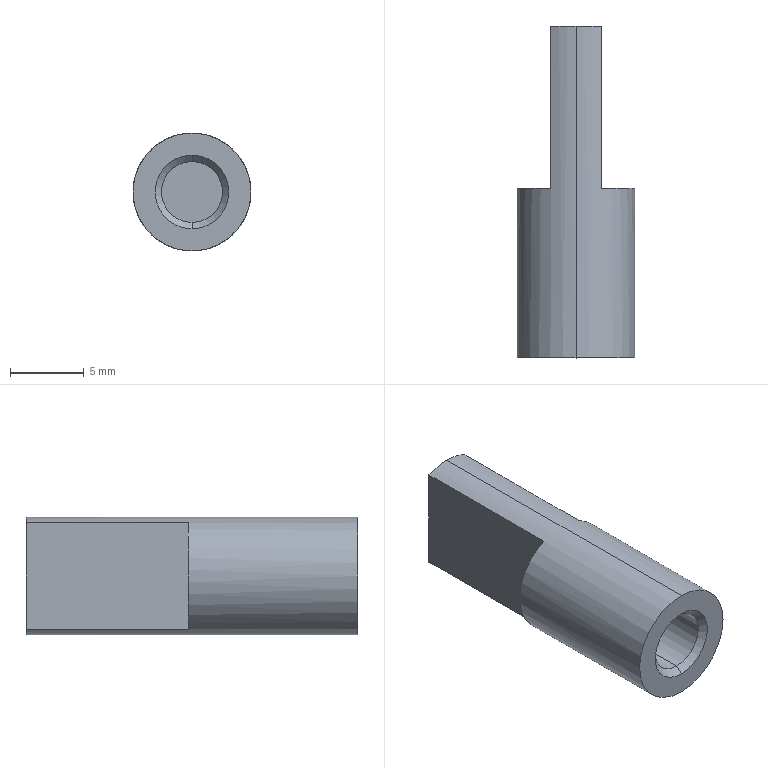Part | STEP file | HI_XAL51-D8-L100-H50-002^XAL51-D8-L100-H50 | 1 solid | 13 faces | box 8 x 22.5 x 8 mm | volume 786.148 mm3 | plane 7 | cylinder 4 | cone 2 | commonest cylinder face diameters 4.134 x2 8 x2
STEP:
#1=CARTESIAN_POINT('',(0.,0.,0.));
#2=DIRECTION('',(0.,0.,1.));
#3=DIRECTION('',(1.,0.,0.));
#4=AXIS2_PLACEMENT_3D('',#1,#2,#3);
#5=CARTESIAN_POINT('',(0.,0.,4.));
#6=VERTEX_POINT('',#5);
#7=CARTESIAN_POINT('',(0.,0.,-4.));
#8=VERTEX_POINT('',#7);
#9=CARTESIAN_POINT('',(0.,0.,0.));
#10=DIRECTION('',(0.,-1.,0.));
#11=DIRECTION('',(0.,0.,-1.));
#12=AXIS2_PLACEMENT_3D('',#9,#10,#11);
#13=CIRCLE('',#12,4.);
#14=CARTESIAN_POINT('',(0.,0.,0.));
#15=DIRECTION('',(0.,1.,0.));
#16=DIRECTION('',(0.,0.,-1.));
#17=AXIS2_PLACEMENT_3D('',#14,#15,#16);
#18=CYLINDRICAL_SURFACE('',#17,4.);
#19=CARTESIAN_POINT('',(6.283,0.));
#20=DIRECTION('',(-1.,0.));
#21=VECTOR('',#20,1.);
#22=LINE('',#19,#21);
#23=(GEOMETRIC_REPRESENTATION_CONTEXT(2)PARAMETRIC_REPRESENTATION_CONTEXT()REPRESENTATION_CONTEXT('',''));
#24=DEFINITIONAL_REPRESENTATION('',(#22),#23);
#25=PCURVE('',#18,#24);
#26=CARTESIAN_POINT('',(4.,0.,0.));
#27=DIRECTION('',(0.,1.,0.));
#28=DIRECTION('',(1.,0.,0.));
#29=AXIS2_PLACEMENT_3D('',#26,#27,#28);
#30=PLANE('',#29);
#31=CARTESIAN_POINT('',(-4.,4.));
#32=CARTESIAN_POINT('',(2.928,4.));
#33=CARTESIAN_POINT('',(-0.5359,-2.));
#34=CARTESIAN_POINT('',(-4.,-8.));
#35=CARTESIAN_POINT('',(-7.464,-2.));
#36=CARTESIAN_POINT('',(-10.928,4.));
#37=CARTESIAN_POINT('',(-4.,4.));
#38=(BOUNDED_CURVE()B_SPLINE_CURVE(2,(#31,#32,#33,#34,#35,#36,#37),.UNSPECIFIED.,.T.,.F.)B_SPLINE_CURVE_WITH_KNOTS((1,2,2,2,2,1),(-2.094,0.,2.094,4.189,6.283,8.378),.UNSPECIFIED.)CURVE()GEOMETRIC_REPRESENTATION_ITEM()RATIONAL_B_SPLINE_CURVE((1.,0.5,1.,0.5,1.,0.5,1.))REPRESENTATION_ITEM(''));
#39=(GEOMETRIC_REPRESENTATION_CONTEXT(2)PARAMETRIC_REPRESENTATION_CONTEXT()REPRESENTATION_CONTEXT('',''));
#40=DEFINITIONAL_REPRESENTATION('',(#38),#39);
#41=PCURVE('',#30,#40);
#42=SURFACE_CURVE('',#13,(#25,#41),.PCURVE_S1.);
#43=EDGE_CURVE('',#6,#8,#42,.T.);
#44=ORIENTED_EDGE('',*,*,#43,.F.);
#45=CARTESIAN_POINT('',(0.,22.5,4.));
#46=VERTEX_POINT('',#45);
#47=CARTESIAN_POINT('',(0.,0.,4.));
#48=DIRECTION('',(0.,1.,0.));
#49=VECTOR('',#48,1.);
#50=LINE('',#47,#49);
#51=CARTESIAN_POINT('',(3.142,0.));
#52=DIRECTION('',(0.,1.));
#53=VECTOR('',#52,1.);
#54=LINE('',#51,#53);
#55=(GEOMETRIC_REPRESENTATION_CONTEXT(2)PARAMETRIC_REPRESENTATION_CONTEXT()REPRESENTATION_CONTEXT('',''));
#56=DEFINITIONAL_REPRESENTATION('',(#54),#55);
#57=PCURVE('',#18,#56);
#58=CARTESIAN_POINT('',(0.,0.,0.));
#59=DIRECTION('',(0.,1.,0.));
#60=DIRECTION('',(0.,0.,-1.));
#61=AXIS2_PLACEMENT_3D('',#58,#59,#60);
#62=CYLINDRICAL_SURFACE('',#61,4.);
#63=CARTESIAN_POINT('',(3.142,0.));
#64=DIRECTION('',(0.,1.));
#65=VECTOR('',#64,1.);
#66=LINE('',#63,#65);
#67=(GEOMETRIC_REPRESENTATION_CONTEXT(2)PARAMETRIC_REPRESENTATION_CONTEXT()REPRESENTATION_CONTEXT('',''));
#68=DEFINITIONAL_REPRESENTATION('',(#66),#67);
#69=PCURVE('',#62,#68);
#70=SURFACE_CURVE('',#50,(#57,#69),.PCURVE_S1.);
#71=EDGE_CURVE('',#6,#46,#70,.T.);
#72=ORIENTED_EDGE('',*,*,#71,.T.);
#73=CARTESIAN_POINT('',(-1.7,22.5,3.621));
#74=VERTEX_POINT('',#73);
#75=CARTESIAN_POINT('',(0.,22.5,0.));
#76=DIRECTION('',(0.,-1.,0.));
#77=DIRECTION('',(0.,0.,-1.));
#78=AXIS2_PLACEMENT_3D('',#75,#76,#77);
#79=CIRCLE('',#78,4.);
#80=CARTESIAN_POINT('',(6.283,22.5));
#81=DIRECTION('',(-1.,0.));
#82=VECTOR('',#81,1.);
#83=LINE('',#80,#82);
#84=(GEOMETRIC_REPRESENTATION_CONTEXT(2)PARAMETRIC_REPRESENTATION_CONTEXT()REPRESENTATION_CONTEXT('',''));
#85=DEFINITIONAL_REPRESENTATION('',(#83),#84);
#86=PCURVE('',#18,#85);
#87=CARTESIAN_POINT('',(0.,22.5,0.));
#88=DIRECTION('',(0.,-1.,0.));
#89=DIRECTION('',(0.,0.,-1.));
#90=AXIS2_PLACEMENT_3D('',#87,#88,#89);
#91=PLANE('',#90);
#92=CARTESIAN_POINT('',(0.,0.));
#93=DIRECTION('',(1.,0.));
#94=AXIS2_PLACEMENT_2D('',#92,#93);
#95=CIRCLE('',#94,4.);
#96=(GEOMETRIC_REPRESENTATION_CONTEXT(2)PARAMETRIC_REPRESENTATION_CONTEXT()REPRESENTATION_CONTEXT('',''));
#97=DEFINITIONAL_REPRESENTATION('',(#95),#96);
#98=PCURVE('',#91,#97);
#99=SURFACE_CURVE('',#79,(#86,#98),.PCURVE_S1.);
#100=EDGE_CURVE('',#46,#74,#99,.T.);
#101=ORIENTED_EDGE('',*,*,#100,.T.);
#102=CARTESIAN_POINT('',(-1.7,11.5,3.621));
#103=VERTEX_POINT('',#102);
#104=CARTESIAN_POINT('',(-1.7,0.,3.621));
#105=DIRECTION('',(0.,1.,0.));
#106=VECTOR('',#105,1.);
#107=LINE('',#104,#106);
#108=CARTESIAN_POINT('',(2.703,0.));
#109=DIRECTION('',(0.,1.));
#110=VECTOR('',#109,1.);
#111=LINE('',#108,#110);
#112=(GEOMETRIC_REPRESENTATION_CONTEXT(2)PARAMETRIC_REPRESENTATION_CONTEXT()REPRESENTATION_CONTEXT('',''));
#113=DEFINITIONAL_REPRESENTATION('',(#111),#112);
#114=PCURVE('',#18,#113);
#115=CARTESIAN_POINT('',(-1.7,11.5,8.));
#116=DIRECTION('',(-1.,0.,0.));
#117=DIRECTION('',(0.,0.,1.));
#118=AXIS2_PLACEMENT_3D('',#115,#116,#117);
#119=PLANE('',#118);
#120=CARTESIAN_POINT('',(-4.379,-11.5));
#121=DIRECTION('',(0.,1.));
#122=VECTOR('',#121,1.);
#123=LINE('',#120,#122);
#124=(GEOMETRIC_REPRESENTATION_CONTEXT(2)PARAMETRIC_REPRESENTATION_CONTEXT()REPRESENTATION_CONTEXT('',''));
#125=DEFINITIONAL_REPRESENTATION('',(#123),#124);
#126=PCURVE('',#119,#125);
#127=SURFACE_CURVE('',#107,(#114,#126),.PCURVE_S1.);
#128=EDGE_CURVE('',#103,#74,#127,.T.);
#129=ORIENTED_EDGE('',*,*,#128,.F.);
#130=CARTESIAN_POINT('',(-1.7,11.5,-3.621));
#131=VERTEX_POINT('',#130);
#132=CARTESIAN_POINT('',(0.,11.5,0.));
#133=DIRECTION('',(0.,1.,0.));
#134=DIRECTION('',(0.,0.,1.));
#135=AXIS2_PLACEMENT_3D('',#132,#133,#134);
#136=CIRCLE('',#135,4.);
#137=CARTESIAN_POINT('',(-3.142,11.5));
#138=DIRECTION('',(1.,0.));
#139=VECTOR('',#138,1.);
#140=LINE('',#137,#139);
#141=(GEOMETRIC_REPRESENTATION_CONTEXT(2)PARAMETRIC_REPRESENTATION_CONTEXT()REPRESENTATION_CONTEXT('',''));
#142=DEFINITIONAL_REPRESENTATION('',(#140),#141);
#143=PCURVE('',#18,#142);
#144=CARTESIAN_POINT('',(-9.7,11.5,8.));
#145=DIRECTION('',(0.,1.,0.));
#146=DIRECTION('',(1.,0.,0.));
#147=AXIS2_PLACEMENT_3D('',#144,#145,#146);
#148=PLANE('',#147);
#149=CARTESIAN_POINT('',(9.7,8.));
#150=DIRECTION('',(0.,-1.));
#151=AXIS2_PLACEMENT_2D('',#149,#150);
#152=CIRCLE('',#151,4.);
#153=(GEOMETRIC_REPRESENTATION_CONTEXT(2)PARAMETRIC_REPRESENTATION_CONTEXT()REPRESENTATION_CONTEXT('',''));
#154=DEFINITIONAL_REPRESENTATION('',(#152),#153);
#155=PCURVE('',#148,#154);
#156=SURFACE_CURVE('',#136,(#143,#155),.PCURVE_S1.);
#157=EDGE_CURVE('',#131,#103,#156,.T.);
#158=ORIENTED_EDGE('',*,*,#157,.F.);
#159=CARTESIAN_POINT('',(-1.7,22.5,-3.621));
#160=VERTEX_POINT('',#159);
#161=CARTESIAN_POINT('',(-1.7,0.,-3.621));
#162=DIRECTION('',(0.,-1.,0.));
#163=VECTOR('',#162,1.);
#164=LINE('',#161,#163);
#165=CARTESIAN_POINT('',(0.439,0.));
#166=DIRECTION('',(0.,-1.));
#167=VECTOR('',#166,1.);
#168=LINE('',#165,#167);
#169=(GEOMETRIC_REPRESENTATION_CONTEXT(2)PARAMETRIC_REPRESENTATION_CONTEXT()REPRESENTATION_CONTEXT('',''));
#170=DEFINITIONAL_REPRESENTATION('',(#168),#169);
#171=PCURVE('',#18,#170);
#172=CARTESIAN_POINT('',(-11.621,-11.5));
#173=DIRECTION('',(0.,-1.));
#174=VECTOR('',#173,1.);
#175=LINE('',#172,#174);
#176=(GEOMETRIC_REPRESENTATION_CONTEXT(2)PARAMETRIC_REPRESENTATION_CONTEXT()REPRESENTATION_CONTEXT('',''));
#177=DEFINITIONAL_REPRESENTATION('',(#175),#176);
#178=PCURVE('',#119,#177);
#179=SURFACE_CURVE('',#164,(#171,#178),.PCURVE_S1.);
#180=EDGE_CURVE('',#160,#131,#179,.T.);
#181=ORIENTED_EDGE('',*,*,#180,.F.);
#182=CARTESIAN_POINT('',(0.,22.5,-4.));
#183=VERTEX_POINT('',#182);
#184=CARTESIAN_POINT('',(0.,22.5,0.));
#185=DIRECTION('',(0.,-1.,0.));
#186=DIRECTION('',(0.,0.,-1.));
#187=AXIS2_PLACEMENT_3D('',#184,#185,#186);
#188=CIRCLE('',#187,4.);
#189=CARTESIAN_POINT('',(6.283,22.5));
#190=DIRECTION('',(-1.,0.));
#191=VECTOR('',#190,1.);
#192=LINE('',#189,#191);
#193=(GEOMETRIC_REPRESENTATION_CONTEXT(2)PARAMETRIC_REPRESENTATION_CONTEXT()REPRESENTATION_CONTEXT('',''));
#194=DEFINITIONAL_REPRESENTATION('',(#192),#193);
#195=PCURVE('',#18,#194);
#196=CARTESIAN_POINT('',(0.,0.));
#197=DIRECTION('',(1.,0.));
#198=AXIS2_PLACEMENT_2D('',#196,#197);
#199=CIRCLE('',#198,4.);
#200=(GEOMETRIC_REPRESENTATION_CONTEXT(2)PARAMETRIC_REPRESENTATION_CONTEXT()REPRESENTATION_CONTEXT('',''));
#201=DEFINITIONAL_REPRESENTATION('',(#199),#200);
#202=PCURVE('',#91,#201);
#203=SURFACE_CURVE('',#188,(#195,#202),.PCURVE_S1.);
#204=EDGE_CURVE('',#160,#183,#203,.T.);
#205=ORIENTED_EDGE('',*,*,#204,.T.);
#206=CARTESIAN_POINT('',(0.,0.,-4.));
#207=DIRECTION('',(0.,1.,0.));
#208=VECTOR('',#207,1.);
#209=LINE('',#206,#208);
#210=CARTESIAN_POINT('',(0.,0.));
#211=DIRECTION('',(0.,1.));
#212=VECTOR('',#211,1.);
#213=LINE('',#210,#212);
#214=(GEOMETRIC_REPRESENTATION_CONTEXT(2)PARAMETRIC_REPRESENTATION_CONTEXT()REPRESENTATION_CONTEXT('',''));
#215=DEFINITIONAL_REPRESENTATION('',(#213),#214);
#216=PCURVE('',#18,#215);
#217=CARTESIAN_POINT('',(6.283,0.));
#218=DIRECTION('',(0.,1.));
#219=VECTOR('',#218,1.);
#220=LINE('',#217,#219);
#221=(GEOMETRIC_REPRESENTATION_CONTEXT(2)PARAMETRIC_REPRESENTATION_CONTEXT()REPRESENTATION_CONTEXT('',''));
#222=DEFINITIONAL_REPRESENTATION('',(#220),#221);
#223=PCURVE('',#62,#222);
#224=SURFACE_CURVE('',#209,(#216,#223),.PCURVE_S1.);
#225=EDGE_CURVE('',#8,#183,#224,.T.);
#226=ORIENTED_EDGE('',*,*,#225,.F.);
#227=EDGE_LOOP('',(#44,#72,#101,#129,#158,#181,#205,#226));
#228=FACE_BOUND('',#227,.T.);
#229=ADVANCED_FACE('',(#228),#18,.T.);
#230=CARTESIAN_POINT('',(0.,0.433,-2.067));
#231=VERTEX_POINT('',#230);
#232=CARTESIAN_POINT('',(0.,0.,-2.5));
#233=VERTEX_POINT('',#232);
#234=CARTESIAN_POINT('',(0.,0.433,-2.067));
#235=DIRECTION('',(0.,-0.7071,-0.7071));
#236=VECTOR('',#235,1.);
#237=LINE('',#234,#236);
#238=CARTESIAN_POINT('',(0.,0.433,0.));
#239=DIRECTION('',(0.,-1.,0.));
#240=DIRECTION('',(0.,0.,-1.));
#241=AXIS2_PLACEMENT_3D('',#238,#239,#240);
#242=CONICAL_SURFACE('',#241,2.067,0.7854);
#243=CARTESIAN_POINT('',(6.283,0.));
#244=DIRECTION('',(0.,1.));
#245=VECTOR('',#244,1.);
#246=LINE('',#243,#245);
#247=(GEOMETRIC_REPRESENTATION_CONTEXT(2)PARAMETRIC_REPRESENTATION_CONTEXT()REPRESENTATION_CONTEXT('',''));
#248=DEFINITIONAL_REPRESENTATION('',(#246),#247);
#249=PCURVE('',#242,#248);
#250=CARTESIAN_POINT('',(0.,0.433,0.));
#251=DIRECTION('',(0.,-1.,0.));
#252=DIRECTION('',(0.,0.,-1.));
#253=AXIS2_PLACEMENT_3D('',#250,#251,#252);
#254=CONICAL_SURFACE('',#253,2.067,0.7854);
#255=CARTESIAN_POINT('',(0.,0.));
#256=DIRECTION('',(0.,1.));
#257=VECTOR('',#256,1.);
#258=LINE('',#255,#257);
#259=(GEOMETRIC_REPRESENTATION_CONTEXT(2)PARAMETRIC_REPRESENTATION_CONTEXT()REPRESENTATION_CONTEXT('',''));
#260=DEFINITIONAL_REPRESENTATION('',(#258),#259);
#261=PCURVE('',#254,#260);
#262=SURFACE_CURVE('',#237,(#249,#261),.PCURVE_S1.);
#263=EDGE_CURVE('',#231,#233,#262,.T.);
#264=ORIENTED_EDGE('',*,*,#263,.T.);
#265=CARTESIAN_POINT('',(0.,0.,2.5));
#266=VERTEX_POINT('',#265);
#267=CARTESIAN_POINT('',(0.,0.,0.));
#268=DIRECTION('',(0.,-1.,0.));
#269=DIRECTION('',(0.,0.,-1.));
#270=AXIS2_PLACEMENT_3D('',#267,#268,#269);
#271=CIRCLE('',#270,2.5);
#272=CARTESIAN_POINT('',(0.,0.433));
#273=DIRECTION('',(1.,0.));
#274=VECTOR('',#273,1.);
#275=LINE('',#272,#274);
#276=(GEOMETRIC_REPRESENTATION_CONTEXT(2)PARAMETRIC_REPRESENTATION_CONTEXT()REPRESENTATION_CONTEXT('',''));
#277=DEFINITIONAL_REPRESENTATION('',(#275),#276);
#278=PCURVE('',#242,#277);
#279=CARTESIAN_POINT('',(-4.,2.5));
#280=CARTESIAN_POINT('',(0.3301,2.5));
#281=CARTESIAN_POINT('',(-1.835,-1.25));
#282=CARTESIAN_POINT('',(-4.,-5.));
#283=CARTESIAN_POINT('',(-6.165,-1.25));
#284=CARTESIAN_POINT('',(-8.33,2.5));
#285=CARTESIAN_POINT('',(-4.,2.5));
#286=(BOUNDED_CURVE()B_SPLINE_CURVE(2,(#279,#280,#281,#282,#283,#284,#285),.UNSPECIFIED.,.T.,.F.)B_SPLINE_CURVE_WITH_KNOTS((1,2,2,2,2,1),(-2.094,0.,2.094,4.189,6.283,8.378),.UNSPECIFIED.)CURVE()GEOMETRIC_REPRESENTATION_ITEM()RATIONAL_B_SPLINE_CURVE((1.,0.5,1.,0.5,1.,0.5,1.))REPRESENTATION_ITEM(''));
#287=(GEOMETRIC_REPRESENTATION_CONTEXT(2)PARAMETRIC_REPRESENTATION_CONTEXT()REPRESENTATION_CONTEXT('',''));
#288=DEFINITIONAL_REPRESENTATION('',(#286),#287);
#289=PCURVE('',#30,#288);
#290=SURFACE_CURVE('',#271,(#278,#289),.PCURVE_S1.);
#291=EDGE_CURVE('',#266,#233,#290,.T.);
#292=ORIENTED_EDGE('',*,*,#291,.F.);
#293=CARTESIAN_POINT('',(0.,0.433,2.067));
#294=VERTEX_POINT('',#293);
#295=CARTESIAN_POINT('',(0.,0.433,2.067));
#296=DIRECTION('',(0.,-0.7071,0.7071));
#297=VECTOR('',#296,1.);
#298=LINE('',#295,#297);
#299=CARTESIAN_POINT('',(3.142,0.));
#300=DIRECTION('',(0.,1.));
#301=VECTOR('',#300,1.);
#302=LINE('',#299,#301);
#303=(GEOMETRIC_REPRESENTATION_CONTEXT(2)PARAMETRIC_REPRESENTATION_CONTEXT()REPRESENTATION_CONTEXT('',''));
#304=DEFINITIONAL_REPRESENTATION('',(#302),#303);
#305=PCURVE('',#242,#304);
#306=CARTESIAN_POINT('',(3.142,0.));
#307=DIRECTION('',(0.,1.));
#308=VECTOR('',#307,1.);
#309=LINE('',#306,#308);
#310=(GEOMETRIC_REPRESENTATION_CONTEXT(2)PARAMETRIC_REPRESENTATION_CONTEXT()REPRESENTATION_CONTEXT('',''));
#311=DEFINITIONAL_REPRESENTATION('',(#309),#310);
#312=PCURVE('',#254,#311);
#313=SURFACE_CURVE('',#298,(#305,#312),.PCURVE_S1.);
#314=EDGE_CURVE('',#294,#266,#313,.T.);
#315=ORIENTED_EDGE('',*,*,#314,.F.);
#316=CARTESIAN_POINT('',(0.,0.433,0.));
#317=DIRECTION('',(0.,-1.,0.));
#318=DIRECTION('',(0.,0.,-1.));
#319=AXIS2_PLACEMENT_3D('',#316,#317,#318);
#320=CIRCLE('',#319,2.067);
#321=CARTESIAN_POINT('',(0.,0.));
#322=DIRECTION('',(1.,0.));
#323=VECTOR('',#322,1.);
#324=LINE('',#321,#323);
#325=(GEOMETRIC_REPRESENTATION_CONTEXT(2)PARAMETRIC_REPRESENTATION_CONTEXT()REPRESENTATION_CONTEXT('',''));
#326=DEFINITIONAL_REPRESENTATION('',(#324),#325);
#327=PCURVE('',#242,#326);
#328=CARTESIAN_POINT('',(0.,0.,0.));
#329=DIRECTION('',(0.,1.,0.));
#330=DIRECTION('',(0.,0.,-1.));
#331=AXIS2_PLACEMENT_3D('',#328,#329,#330);
#332=CYLINDRICAL_SURFACE('',#331,2.067);
#333=CARTESIAN_POINT('',(6.283,0.433));
#334=DIRECTION('',(-1.,0.));
#335=VECTOR('',#334,1.);
#336=LINE('',#333,#335);
#337=(GEOMETRIC_REPRESENTATION_CONTEXT(2)PARAMETRIC_REPRESENTATION_CONTEXT()REPRESENTATION_CONTEXT('',''));
#338=DEFINITIONAL_REPRESENTATION('',(#336),#337);
#339=PCURVE('',#332,#338);
#340=SURFACE_CURVE('',#320,(#327,#339),.PCURVE_S1.);
#341=EDGE_CURVE('',#294,#231,#340,.T.);
#342=ORIENTED_EDGE('',*,*,#341,.T.);
#343=EDGE_LOOP('',(#264,#292,#315,#342));
#344=FACE_BOUND('',#343,.F.);
#345=ADVANCED_FACE('',(#344),#242,.F.);
#346=CARTESIAN_POINT('',(0.,6.,-2.067));
#347=VERTEX_POINT('',#346);
#348=CARTESIAN_POINT('',(0.,0.,-2.067));
#349=DIRECTION('',(0.,1.,0.));
#350=VECTOR('',#349,1.);
#351=LINE('',#348,#350);
#352=CARTESIAN_POINT('',(0.,0.,0.));
#353=DIRECTION('',(0.,1.,0.));
#354=DIRECTION('',(0.,0.,-1.));
#355=AXIS2_PLACEMENT_3D('',#352,#353,#354);
#356=CYLINDRICAL_SURFACE('',#355,2.067);
#357=CARTESIAN_POINT('',(6.283,0.));
#358=DIRECTION('',(0.,1.));
#359=VECTOR('',#358,1.);
#360=LINE('',#357,#359);
#361=(GEOMETRIC_REPRESENTATION_CONTEXT(2)PARAMETRIC_REPRESENTATION_CONTEXT()REPRESENTATION_CONTEXT('',''));
#362=DEFINITIONAL_REPRESENTATION('',(#360),#361);
#363=PCURVE('',#356,#362);
#364=CARTESIAN_POINT('',(0.,0.));
#365=DIRECTION('',(0.,1.));
#366=VECTOR('',#365,1.);
#367=LINE('',#364,#366);
#368=(GEOMETRIC_REPRESENTATION_CONTEXT(2)PARAMETRIC_REPRESENTATION_CONTEXT()REPRESENTATION_CONTEXT('',''));
#369=DEFINITIONAL_REPRESENTATION('',(#367),#368);
#370=PCURVE('',#332,#369);
#371=SURFACE_CURVE('',#351,(#363,#370),.PCURVE_S1.);
#372=EDGE_CURVE('',#231,#347,#371,.T.);
#373=ORIENTED_EDGE('',*,*,#372,.T.);
#374=CARTESIAN_POINT('',(0.,6.,2.067));
#375=VERTEX_POINT('',#374);
#376=CARTESIAN_POINT('',(0.,6.,0.));
#377=DIRECTION('',(0.,-1.,0.));
#378=DIRECTION('',(0.,0.,-1.));
#379=AXIS2_PLACEMENT_3D('',#376,#377,#378);
#380=CIRCLE('',#379,2.067);
#381=CARTESIAN_POINT('',(6.283,6.));
#382=DIRECTION('',(-1.,0.));
#383=VECTOR('',#382,1.);
#384=LINE('',#381,#383);
#385=(GEOMETRIC_REPRESENTATION_CONTEXT(2)PARAMETRIC_REPRESENTATION_CONTEXT()REPRESENTATION_CONTEXT('',''));
#386=DEFINITIONAL_REPRESENTATION('',(#384),#385);
#387=PCURVE('',#356,#386);
#388=CARTESIAN_POINT('',(0.,6.,0.));
#389=DIRECTION('',(0.,-1.,0.));
#390=DIRECTION('',(0.,0.,-1.));
#391=AXIS2_PLACEMENT_3D('',#388,#389,#390);
#392=PLANE('',#391);
#393=CARTESIAN_POINT('',(0.,0.));
#394=DIRECTION('',(1.,0.));
#395=AXIS2_PLACEMENT_2D('',#393,#394);
#396=CIRCLE('',#395,2.067);
#397=(GEOMETRIC_REPRESENTATION_CONTEXT(2)PARAMETRIC_REPRESENTATION_CONTEXT()REPRESENTATION_CONTEXT('',''));
#398=DEFINITIONAL_REPRESENTATION('',(#396),#397);
#399=PCURVE('',#392,#398);
#400=SURFACE_CURVE('',#380,(#387,#399),.PCURVE_S1.);
#401=EDGE_CURVE('',#347,#375,#400,.T.);
#402=ORIENTED_EDGE('',*,*,#401,.T.);
#403=CARTESIAN_POINT('',(0.,0.,2.067));
#404=DIRECTION('',(0.,1.,0.));
#405=VECTOR('',#404,1.);
#406=LINE('',#403,#405);
#407=CARTESIAN_POINT('',(3.142,0.));
#408=DIRECTION('',(0.,1.));
#409=VECTOR('',#408,1.);
#410=LINE('',#407,#409);
#411=(GEOMETRIC_REPRESENTATION_CONTEXT(2)PARAMETRIC_REPRESENTATION_CONTEXT()REPRESENTATION_CONTEXT('',''));
#412=DEFINITIONAL_REPRESENTATION('',(#410),#411);
#413=PCURVE('',#356,#412);
#414=CARTESIAN_POINT('',(3.142,0.));
#415=DIRECTION('',(0.,1.));
#416=VECTOR('',#415,1.);
#417=LINE('',#414,#416);
#418=(GEOMETRIC_REPRESENTATION_CONTEXT(2)PARAMETRIC_REPRESENTATION_CONTEXT()REPRESENTATION_CONTEXT('',''));
#419=DEFINITIONAL_REPRESENTATION('',(#417),#418);
#420=PCURVE('',#332,#419);
#421=SURFACE_CURVE('',#406,(#413,#420),.PCURVE_S1.);
#422=EDGE_CURVE('',#294,#375,#421,.T.);
#423=ORIENTED_EDGE('',*,*,#422,.F.);
#424=CARTESIAN_POINT('',(0.,0.433,0.));
#425=DIRECTION('',(0.,-1.,0.));
#426=DIRECTION('',(0.,0.,-1.));
#427=AXIS2_PLACEMENT_3D('',#424,#425,#426);
#428=CIRCLE('',#427,2.067);
#429=CARTESIAN_POINT('',(6.283,0.433));
#430=DIRECTION('',(-1.,0.));
#431=VECTOR('',#430,1.);
#432=LINE('',#429,#431);
#433=(GEOMETRIC_REPRESENTATION_CONTEXT(2)PARAMETRIC_REPRESENTATION_CONTEXT()REPRESENTATION_CONTEXT('',''));
#434=DEFINITIONAL_REPRESENTATION('',(#432),#433);
#435=PCURVE('',#356,#434);
#436=CARTESIAN_POINT('',(0.,0.));
#437=DIRECTION('',(1.,0.));
#438=VECTOR('',#437,1.);
#439=LINE('',#436,#438);
#440=(GEOMETRIC_REPRESENTATION_CONTEXT(2)PARAMETRIC_REPRESENTATION_CONTEXT()REPRESENTATION_CONTEXT('',''));
#441=DEFINITIONAL_REPRESENTATION('',(#439),#440);
#442=PCURVE('',#254,#441);
#443=SURFACE_CURVE('',#428,(#435,#442),.PCURVE_S1.);
#444=EDGE_CURVE('',#231,#294,#443,.T.);
#445=ORIENTED_EDGE('',*,*,#444,.F.);
#446=EDGE_LOOP('',(#373,#402,#423,#445));
#447=FACE_BOUND('',#446,.F.);
#448=ADVANCED_FACE('',(#447),#356,.F.);
#449=ORIENTED_EDGE('',*,*,#401,.T.);
#450=CARTESIAN_POINT('',(0.,6.,0.));
#451=DIRECTION('',(0.,-1.,0.));
#452=DIRECTION('',(0.,0.,-1.));
#453=AXIS2_PLACEMENT_3D('',#450,#451,#452);
#454=CIRCLE('',#453,2.067);
#455=CARTESIAN_POINT('',(0.,0.));
#456=DIRECTION('',(1.,0.));
#457=AXIS2_PLACEMENT_2D('',#455,#456);
#458=CIRCLE('',#457,2.067);
#459=(GEOMETRIC_REPRESENTATION_CONTEXT(2)PARAMETRIC_REPRESENTATION_CONTEXT()REPRESENTATION_CONTEXT('',''));
#460=DEFINITIONAL_REPRESENTATION('',(#458),#459);
#461=PCURVE('',#392,#460);
#462=CARTESIAN_POINT('',(6.283,6.));
#463=DIRECTION('',(-1.,0.));
#464=VECTOR('',#463,1.);
#465=LINE('',#462,#464);
#466=(GEOMETRIC_REPRESENTATION_CONTEXT(2)PARAMETRIC_REPRESENTATION_CONTEXT()REPRESENTATION_CONTEXT('',''));
#467=DEFINITIONAL_REPRESENTATION('',(#465),#466);
#468=PCURVE('',#332,#467);
#469=SURFACE_CURVE('',#454,(#461,#468),.PCURVE_S1.);
#470=EDGE_CURVE('',#375,#347,#469,.T.);
#471=ORIENTED_EDGE('',*,*,#470,.T.);
#472=EDGE_LOOP('',(#449,#471));
#473=FACE_BOUND('',#472,.T.);
#474=ADVANCED_FACE('',(#473),#392,.T.);
#475=CARTESIAN_POINT('',(0.,0.,0.));
#476=DIRECTION('',(0.,-1.,0.));
#477=DIRECTION('',(0.,0.,-1.));
#478=AXIS2_PLACEMENT_3D('',#475,#476,#477);
#479=CIRCLE('',#478,2.5);
#480=CARTESIAN_POINT('',(-4.,2.5));
#481=CARTESIAN_POINT('',(0.3301,2.5));
#482=CARTESIAN_POINT('',(-1.835,-1.25));
#483=CARTESIAN_POINT('',(-4.,-5.));
#484=CARTESIAN_POINT('',(-6.165,-1.25));
#485=CARTESIAN_POINT('',(-8.33,2.5));
#486=CARTESIAN_POINT('',(-4.,2.5));
#487=(BOUNDED_CURVE()B_SPLINE_CURVE(2,(#480,#481,#482,#483,#484,#485,#486),.UNSPECIFIED.,.T.,.F.)B_SPLINE_CURVE_WITH_KNOTS((1,2,2,2,2,1),(-2.094,0.,2.094,4.189,6.283,8.378),.UNSPECIFIED.)CURVE()GEOMETRIC_REPRESENTATION_ITEM()RATIONAL_B_SPLINE_CURVE((1.,0.5,1.,0.5,1.,0.5,1.))REPRESENTATION_ITEM(''));
#488=(GEOMETRIC_REPRESENTATION_CONTEXT(2)PARAMETRIC_REPRESENTATION_CONTEXT()REPRESENTATION_CONTEXT('',''));
#489=DEFINITIONAL_REPRESENTATION('',(#487),#488);
#490=PCURVE('',#30,#489);
#491=CARTESIAN_POINT('',(0.,0.433));
#492=DIRECTION('',(1.,0.));
#493=VECTOR('',#492,1.);
#494=LINE('',#491,#493);
#495=(GEOMETRIC_REPRESENTATION_CONTEXT(2)PARAMETRIC_REPRESENTATION_CONTEXT()REPRESENTATION_CONTEXT('',''));
#496=DEFINITIONAL_REPRESENTATION('',(#494),#495);
#497=PCURVE('',#254,#496);
#498=SURFACE_CURVE('',#479,(#490,#497),.PCURVE_S1.);
#499=EDGE_CURVE('',#233,#266,#498,.T.);
#500=ORIENTED_EDGE('',*,*,#499,.F.);
#501=ORIENTED_EDGE('',*,*,#291,.F.);
#502=EDGE_LOOP('',(#500,#501));
#503=FACE_BOUND('',#502,.T.);
#504=CARTESIAN_POINT('',(0.,0.,0.));
#505=DIRECTION('',(0.,-1.,0.));
#506=DIRECTION('',(0.,0.,-1.));
#507=AXIS2_PLACEMENT_3D('',#504,#505,#506);
#508=CIRCLE('',#507,4.);
#509=CARTESIAN_POINT('',(-4.,4.));
#510=CARTESIAN_POINT('',(2.928,4.));
#511=CARTESIAN_POINT('',(-0.5359,-2.));
#512=CARTESIAN_POINT('',(-4.,-8.));
#513=CARTESIAN_POINT('',(-7.464,-2.));
#514=CARTESIAN_POINT('',(-10.928,4.));
#515=CARTESIAN_POINT('',(-4.,4.));
#516=(BOUNDED_CURVE()B_SPLINE_CURVE(2,(#509,#510,#511,#512,#513,#514,#515),.UNSPECIFIED.,.T.,.F.)B_SPLINE_CURVE_WITH_KNOTS((1,2,2,2,2,1),(-2.094,0.,2.094,4.189,6.283,8.378),.UNSPECIFIED.)CURVE()GEOMETRIC_REPRESENTATION_ITEM()RATIONAL_B_SPLINE_CURVE((1.,0.5,1.,0.5,1.,0.5,1.))REPRESENTATION_ITEM(''));
#517=(GEOMETRIC_REPRESENTATION_CONTEXT(2)PARAMETRIC_REPRESENTATION_CONTEXT()REPRESENTATION_CONTEXT('',''));
#518=DEFINITIONAL_REPRESENTATION('',(#516),#517);
#519=PCURVE('',#30,#518);
#520=CARTESIAN_POINT('',(6.283,0.));
#521=DIRECTION('',(-1.,0.));
#522=VECTOR('',#521,1.);
#523=LINE('',#520,#522);
#524=(GEOMETRIC_REPRESENTATION_CONTEXT(2)PARAMETRIC_REPRESENTATION_CONTEXT()REPRESENTATION_CONTEXT('',''));
#525=DEFINITIONAL_REPRESENTATION('',(#523),#524);
#526=PCURVE('',#62,#525);
#527=SURFACE_CURVE('',#508,(#519,#526),.PCURVE_S1.);
#528=EDGE_CURVE('',#8,#6,#527,.T.);
#529=ORIENTED_EDGE('',*,*,#528,.T.);
#530=ORIENTED_EDGE('',*,*,#43,.T.);
#531=EDGE_LOOP('',(#529,#530));
#532=FACE_BOUND('',#531,.T.);
#533=ADVANCED_FACE('',(#503,#532),#30,.F.);
#534=ORIENTED_EDGE('',*,*,#470,.T.);
#535=ORIENTED_EDGE('',*,*,#372,.F.);
#536=ORIENTED_EDGE('',*,*,#341,.F.);
#537=ORIENTED_EDGE('',*,*,#422,.T.);
#538=EDGE_LOOP('',(#534,#535,#536,#537));
#539=FACE_BOUND('',#538,.F.);
#540=ADVANCED_FACE('',(#539),#332,.F.);
#541=ORIENTED_EDGE('',*,*,#499,.F.);
#542=ORIENTED_EDGE('',*,*,#263,.F.);
#543=ORIENTED_EDGE('',*,*,#444,.T.);
#544=ORIENTED_EDGE('',*,*,#314,.T.);
#545=EDGE_LOOP('',(#541,#542,#543,#544));
#546=FACE_BOUND('',#545,.F.);
#547=ADVANCED_FACE('',(#546),#254,.F.);
#548=ORIENTED_EDGE('',*,*,#157,.T.);
#549=CARTESIAN_POINT('',(-1.7,11.5,8.));
#550=DIRECTION('',(0.,0.,-1.));
#551=VECTOR('',#550,1.);
#552=LINE('',#549,#551);
#553=CARTESIAN_POINT('',(8.,0.));
#554=DIRECTION('',(0.,1.));
#555=VECTOR('',#554,1.);
#556=LINE('',#553,#555);
#557=(GEOMETRIC_REPRESENTATION_CONTEXT(2)PARAMETRIC_REPRESENTATION_CONTEXT()REPRESENTATION_CONTEXT('',''));
#558=DEFINITIONAL_REPRESENTATION('',(#556),#557);
#559=PCURVE('',#148,#558);
#560=CARTESIAN_POINT('',(0.,0.));
#561=DIRECTION('',(-1.,0.));
#562=VECTOR('',#561,1.);
#563=LINE('',#560,#562);
#564=(GEOMETRIC_REPRESENTATION_CONTEXT(2)PARAMETRIC_REPRESENTATION_CONTEXT()REPRESENTATION_CONTEXT('',''));
#565=DEFINITIONAL_REPRESENTATION('',(#563),#564);
#566=PCURVE('',#119,#565);
#567=SURFACE_CURVE('',#552,(#559,#566),.PCURVE_S1.);
#568=EDGE_CURVE('',#103,#131,#567,.T.);
#569=ORIENTED_EDGE('',*,*,#568,.T.);
#570=EDGE_LOOP('',(#548,#569));
#571=FACE_BOUND('',#570,.T.);
#572=ADVANCED_FACE('',(#571),#148,.T.);
#573=ORIENTED_EDGE('',*,*,#180,.T.);
#574=ORIENTED_EDGE('',*,*,#568,.F.);
#575=ORIENTED_EDGE('',*,*,#128,.T.);
#576=CARTESIAN_POINT('',(-1.7,22.5,0.));
#577=DIRECTION('',(0.,0.,-1.));
#578=VECTOR('',#577,1.);
#579=LINE('',#576,#578);
#580=CARTESIAN_POINT('',(-8.,11.));
#581=DIRECTION('',(-1.,0.));
#582=VECTOR('',#581,1.);
#583=LINE('',#580,#582);
#584=(GEOMETRIC_REPRESENTATION_CONTEXT(2)PARAMETRIC_REPRESENTATION_CONTEXT()REPRESENTATION_CONTEXT('',''));
#585=DEFINITIONAL_REPRESENTATION('',(#583),#584);
#586=PCURVE('',#119,#585);
#587=CARTESIAN_POINT('',(0.,-1.7));
#588=DIRECTION('',(1.,0.));
#589=VECTOR('',#588,1.);
#590=LINE('',#587,#589);
#591=(GEOMETRIC_REPRESENTATION_CONTEXT(2)PARAMETRIC_REPRESENTATION_CONTEXT()REPRESENTATION_CONTEXT('',''));
#592=DEFINITIONAL_REPRESENTATION('',(#590),#591);
#593=PCURVE('',#91,#592);
#594=SURFACE_CURVE('',#579,(#586,#593),.PCURVE_S1.);
#595=EDGE_CURVE('',#74,#160,#594,.T.);
#596=ORIENTED_EDGE('',*,*,#595,.T.);
#597=EDGE_LOOP('',(#573,#574,#575,#596));
#598=FACE_BOUND('',#597,.T.);
#599=ADVANCED_FACE('',(#598),#119,.T.);
#600=ORIENTED_EDGE('',*,*,#71,.F.);
#601=ORIENTED_EDGE('',*,*,#528,.F.);
#602=ORIENTED_EDGE('',*,*,#225,.T.);
#603=CARTESIAN_POINT('',(1.7,22.5,-3.621));
#604=VERTEX_POINT('',#603);
#605=CARTESIAN_POINT('',(0.,22.5,0.));
#606=DIRECTION('',(0.,-1.,0.));
#607=DIRECTION('',(0.,0.,-1.));
#608=AXIS2_PLACEMENT_3D('',#605,#606,#607);
#609=CIRCLE('',#608,4.);
#610=CARTESIAN_POINT('',(6.283,22.5));
#611=DIRECTION('',(-1.,0.));
#612=VECTOR('',#611,1.);
#613=LINE('',#610,#612);
#614=(GEOMETRIC_REPRESENTATION_CONTEXT(2)PARAMETRIC_REPRESENTATION_CONTEXT()REPRESENTATION_CONTEXT('',''));
#615=DEFINITIONAL_REPRESENTATION('',(#613),#614);
#616=PCURVE('',#62,#615);
#617=CARTESIAN_POINT('',(0.,0.));
#618=DIRECTION('',(1.,0.));
#619=AXIS2_PLACEMENT_2D('',#617,#618);
#620=CIRCLE('',#619,4.);
#621=(GEOMETRIC_REPRESENTATION_CONTEXT(2)PARAMETRIC_REPRESENTATION_CONTEXT()REPRESENTATION_CONTEXT('',''));
#622=DEFINITIONAL_REPRESENTATION('',(#620),#621);
#623=PCURVE('',#91,#622);
#624=SURFACE_CURVE('',#609,(#616,#623),.PCURVE_S1.);
#625=EDGE_CURVE('',#183,#604,#624,.T.);
#626=ORIENTED_EDGE('',*,*,#625,.T.);
#627=CARTESIAN_POINT('',(1.7,11.5,-3.621));
#628=VERTEX_POINT('',#627);
#629=CARTESIAN_POINT('',(1.7,0.,-3.621));
#630=DIRECTION('',(0.,1.,0.));
#631=VECTOR('',#630,1.);
#632=LINE('',#629,#631);
#633=CARTESIAN_POINT('',(5.844,0.));
#634=DIRECTION('',(0.,1.));
#635=VECTOR('',#634,1.);
#636=LINE('',#633,#635);
#637=(GEOMETRIC_REPRESENTATION_CONTEXT(2)PARAMETRIC_REPRESENTATION_CONTEXT()REPRESENTATION_CONTEXT('',''));
#638=DEFINITIONAL_REPRESENTATION('',(#636),#637);
#639=PCURVE('',#62,#638);
#640=CARTESIAN_POINT('',(1.7,29.5,8.));
#641=DIRECTION('',(1.,0.,0.));
#642=DIRECTION('',(0.,-1.,0.));
#643=AXIS2_PLACEMENT_3D('',#640,#641,#642);
#644=PLANE('',#643);
#645=CARTESIAN_POINT('',(29.5,11.621));
#646=DIRECTION('',(-1.,0.));
#647=VECTOR('',#646,1.);
#648=LINE('',#645,#647);
#649=(GEOMETRIC_REPRESENTATION_CONTEXT(2)PARAMETRIC_REPRESENTATION_CONTEXT()REPRESENTATION_CONTEXT('',''));
#650=DEFINITIONAL_REPRESENTATION('',(#648),#649);
#651=PCURVE('',#644,#650);
#652=SURFACE_CURVE('',#632,(#639,#651),.PCURVE_S1.);
#653=EDGE_CURVE('',#628,#604,#652,.T.);
#654=ORIENTED_EDGE('',*,*,#653,.F.);
#655=CARTESIAN_POINT('',(1.7,11.5,3.621));
#656=VERTEX_POINT('',#655);
#657=CARTESIAN_POINT('',(0.,11.5,0.));
#658=DIRECTION('',(0.,1.,0.));
#659=DIRECTION('',(0.,0.,1.));
#660=AXIS2_PLACEMENT_3D('',#657,#658,#659);
#661=CIRCLE('',#660,4.);
#662=CARTESIAN_POINT('',(3.142,11.5));
#663=DIRECTION('',(1.,0.));
#664=VECTOR('',#663,1.);
#665=LINE('',#662,#664);
#666=(GEOMETRIC_REPRESENTATION_CONTEXT(2)PARAMETRIC_REPRESENTATION_CONTEXT()REPRESENTATION_CONTEXT('',''));
#667=DEFINITIONAL_REPRESENTATION('',(#665),#666);
#668=PCURVE('',#62,#667);
#669=CARTESIAN_POINT('',(1.7,11.5,8.));
#670=DIRECTION('',(0.,1.,0.));
#671=DIRECTION('',(1.,0.,0.));
#672=AXIS2_PLACEMENT_3D('',#669,#670,#671);
#673=PLANE('',#672);
#674=CARTESIAN_POINT('',(-1.7,8.));
#675=DIRECTION('',(0.,-1.));
#676=AXIS2_PLACEMENT_2D('',#674,#675);
#677=CIRCLE('',#676,4.);
#678=(GEOMETRIC_REPRESENTATION_CONTEXT(2)PARAMETRIC_REPRESENTATION_CONTEXT()REPRESENTATION_CONTEXT('',''));
#679=DEFINITIONAL_REPRESENTATION('',(#677),#678);
#680=PCURVE('',#673,#679);
#681=SURFACE_CURVE('',#661,(#668,#680),.PCURVE_S1.);
#682=EDGE_CURVE('',#656,#628,#681,.T.);
#683=ORIENTED_EDGE('',*,*,#682,.F.);
#684=CARTESIAN_POINT('',(1.7,22.5,3.621));
#685=VERTEX_POINT('',#684);
#686=CARTESIAN_POINT('',(1.7,0.,3.621));
#687=DIRECTION('',(0.,-1.,0.));
#688=VECTOR('',#687,1.);
#689=LINE('',#686,#688);
#690=CARTESIAN_POINT('',(3.581,0.));
#691=DIRECTION('',(0.,-1.));
#692=VECTOR('',#691,1.);
#693=LINE('',#690,#692);
#694=(GEOMETRIC_REPRESENTATION_CONTEXT(2)PARAMETRIC_REPRESENTATION_CONTEXT()REPRESENTATION_CONTEXT('',''));
#695=DEFINITIONAL_REPRESENTATION('',(#693),#694);
#696=PCURVE('',#62,#695);
#697=CARTESIAN_POINT('',(29.5,4.379));
#698=DIRECTION('',(1.,0.));
#699=VECTOR('',#698,1.);
#700=LINE('',#697,#699);
#701=(GEOMETRIC_REPRESENTATION_CONTEXT(2)PARAMETRIC_REPRESENTATION_CONTEXT()REPRESENTATION_CONTEXT('',''));
#702=DEFINITIONAL_REPRESENTATION('',(#700),#701);
#703=PCURVE('',#644,#702);
#704=SURFACE_CURVE('',#689,(#696,#703),.PCURVE_S1.);
#705=EDGE_CURVE('',#685,#656,#704,.T.);
#706=ORIENTED_EDGE('',*,*,#705,.F.);
#707=CARTESIAN_POINT('',(0.,22.5,0.));
#708=DIRECTION('',(0.,-1.,0.));
#709=DIRECTION('',(0.,0.,-1.));
#710=AXIS2_PLACEMENT_3D('',#707,#708,#709);
#711=CIRCLE('',#710,4.);
#712=CARTESIAN_POINT('',(6.283,22.5));
#713=DIRECTION('',(-1.,0.));
#714=VECTOR('',#713,1.);
#715=LINE('',#712,#714);
#716=(GEOMETRIC_REPRESENTATION_CONTEXT(2)PARAMETRIC_REPRESENTATION_CONTEXT()REPRESENTATION_CONTEXT('',''));
#717=DEFINITIONAL_REPRESENTATION('',(#715),#716);
#718=PCURVE('',#62,#717);
#719=CARTESIAN_POINT('',(0.,0.));
#720=DIRECTION('',(1.,0.));
#721=AXIS2_PLACEMENT_2D('',#719,#720);
#722=CIRCLE('',#721,4.);
#723=(GEOMETRIC_REPRESENTATION_CONTEXT(2)PARAMETRIC_REPRESENTATION_CONTEXT()REPRESENTATION_CONTEXT('',''));
#724=DEFINITIONAL_REPRESENTATION('',(#722),#723);
#725=PCURVE('',#91,#724);
#726=SURFACE_CURVE('',#711,(#718,#725),.PCURVE_S1.);
#727=EDGE_CURVE('',#685,#46,#726,.T.);
#728=ORIENTED_EDGE('',*,*,#727,.T.);
#729=EDGE_LOOP('',(#600,#601,#602,#626,#654,#683,#706,#728));
#730=FACE_BOUND('',#729,.T.);
#731=ADVANCED_FACE('',(#730),#62,.T.);
#732=ORIENTED_EDGE('',*,*,#705,.T.);
#733=CARTESIAN_POINT('',(1.7,11.5,8.));
#734=DIRECTION('',(0.,0.,-1.));
#735=VECTOR('',#734,1.);
#736=LINE('',#733,#735);
#737=CARTESIAN_POINT('',(18.,0.));
#738=DIRECTION('',(0.,1.));
#739=VECTOR('',#738,1.);
#740=LINE('',#737,#739);
#741=(GEOMETRIC_REPRESENTATION_CONTEXT(2)PARAMETRIC_REPRESENTATION_CONTEXT()REPRESENTATION_CONTEXT('',''));
#742=DEFINITIONAL_REPRESENTATION('',(#740),#741);
#743=PCURVE('',#644,#742);
#744=CARTESIAN_POINT('',(0.,0.));
#745=DIRECTION('',(0.,1.));
#746=VECTOR('',#745,1.);
#747=LINE('',#744,#746);
#748=(GEOMETRIC_REPRESENTATION_CONTEXT(2)PARAMETRIC_REPRESENTATION_CONTEXT()REPRESENTATION_CONTEXT('',''));
#749=DEFINITIONAL_REPRESENTATION('',(#747),#748);
#750=PCURVE('',#673,#749);
#751=SURFACE_CURVE('',#736,(#743,#750),.PCURVE_S1.);
#752=EDGE_CURVE('',#656,#628,#751,.T.);
#753=ORIENTED_EDGE('',*,*,#752,.T.);
#754=ORIENTED_EDGE('',*,*,#653,.T.);
#755=CARTESIAN_POINT('',(1.7,22.5,0.));
#756=DIRECTION('',(0.,0.,1.));
#757=VECTOR('',#756,1.);
#758=LINE('',#755,#757);
#759=CARTESIAN_POINT('',(7.,8.));
#760=DIRECTION('',(0.,-1.));
#761=VECTOR('',#760,1.);
#762=LINE('',#759,#761);
#763=(GEOMETRIC_REPRESENTATION_CONTEXT(2)PARAMETRIC_REPRESENTATION_CONTEXT()REPRESENTATION_CONTEXT('',''));
#764=DEFINITIONAL_REPRESENTATION('',(#762),#763);
#765=PCURVE('',#644,#764);
#766=CARTESIAN_POINT('',(0.,1.7));
#767=DIRECTION('',(-1.,0.));
#768=VECTOR('',#767,1.);
#769=LINE('',#766,#768);
#770=(GEOMETRIC_REPRESENTATION_CONTEXT(2)PARAMETRIC_REPRESENTATION_CONTEXT()REPRESENTATION_CONTEXT('',''));
#771=DEFINITIONAL_REPRESENTATION('',(#769),#770);
#772=PCURVE('',#91,#771);
#773=SURFACE_CURVE('',#758,(#765,#772),.PCURVE_S1.);
#774=EDGE_CURVE('',#604,#685,#773,.T.);
#775=ORIENTED_EDGE('',*,*,#774,.T.);
#776=EDGE_LOOP('',(#732,#753,#754,#775));
#777=FACE_BOUND('',#776,.T.);
#778=ADVANCED_FACE('',(#777),#644,.T.);
#779=ORIENTED_EDGE('',*,*,#682,.T.);
#780=ORIENTED_EDGE('',*,*,#752,.F.);
#781=EDGE_LOOP('',(#779,#780));
#782=FACE_BOUND('',#781,.T.);
#783=ADVANCED_FACE('',(#782),#673,.T.);
#784=ORIENTED_EDGE('',*,*,#774,.F.);
#785=ORIENTED_EDGE('',*,*,#625,.F.);
#786=ORIENTED_EDGE('',*,*,#204,.F.);
#787=ORIENTED_EDGE('',*,*,#595,.F.);
#788=ORIENTED_EDGE('',*,*,#100,.F.);
#789=ORIENTED_EDGE('',*,*,#727,.F.);
#790=EDGE_LOOP('',(#784,#785,#786,#787,#788,#789));
#791=FACE_BOUND('',#790,.T.);
#792=ADVANCED_FACE('',(#791),#91,.F.);
#793=CLOSED_SHELL('',(#229,#345,#448,#474,#533,#540,#547,#572,#599,#731,#778,#783,#792));
#794=MANIFOLD_SOLID_BREP('',#793);
#795=(LENGTH_UNIT()NAMED_UNIT(*)SI_UNIT(.MILLI.,.METRE.));
#796=UNCERTAINTY_MEASURE_WITH_UNIT(LENGTH_MEASURE(0.0000001),#795,'','');
#797=(NAMED_UNIT(*)PLANE_ANGLE_UNIT()SI_UNIT($,.RADIAN.));
#798=(NAMED_UNIT(*)SI_UNIT($,.STERADIAN.)SOLID_ANGLE_UNIT());
#799=(GEOMETRIC_REPRESENTATION_CONTEXT(3)GLOBAL_UNCERTAINTY_ASSIGNED_CONTEXT((#796))GLOBAL_UNIT_ASSIGNED_CONTEXT((#795,#797,#798))REPRESENTATION_CONTEXT('',''));
#800=ADVANCED_BREP_SHAPE_REPRESENTATION('',(#4,#794),#799);